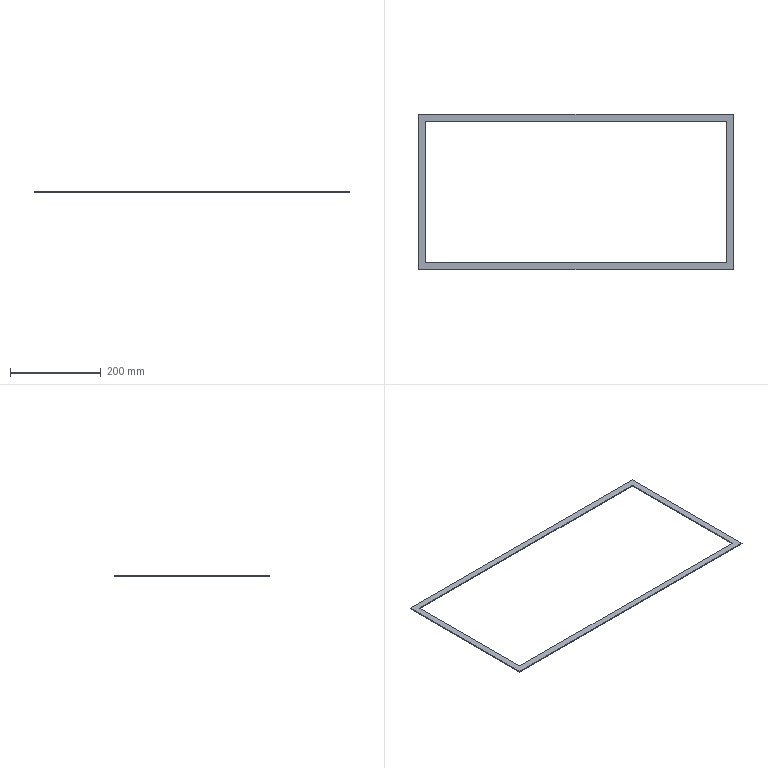Part | SolidWorks | features Extrusion 1 | 1 solid | 10 faces | box 692 x 342 x 2 mm | volume 60240 mm3 | plane 10
STEP:
#1=CARTESIAN_POINT('',(346.,-171.,1.));
#2=VERTEX_POINT('',#1);
#3=CARTESIAN_POINT('',(346.,171.,1.));
#4=VERTEX_POINT('',#3);
#5=CARTESIAN_POINT('',(346.,-171.,1.));
#6=DIRECTION('',(0.,1.,0.));
#7=VECTOR('',#6,1000.);
#8=LINE('',#5,#7);
#9=EDGE_CURVE('',#2,#4,#8,.T.);
#10=ORIENTED_EDGE('',*,*,#9,.T.);
#11=CARTESIAN_POINT('',(-346.,171.,1.));
#12=VERTEX_POINT('',#11);
#13=CARTESIAN_POINT('',(-346.,171.,1.));
#14=DIRECTION('',(-1.,0.,0.));
#15=VECTOR('',#14,1000.);
#16=LINE('',#13,#15);
#17=EDGE_CURVE('',#4,#12,#16,.T.);
#18=ORIENTED_EDGE('',*,*,#17,.T.);
#19=CARTESIAN_POINT('',(-346.,-171.,1.));
#20=VERTEX_POINT('',#19);
#21=CARTESIAN_POINT('',(-346.,-171.,1.));
#22=DIRECTION('',(0.,-1.,0.));
#23=VECTOR('',#22,1000.);
#24=LINE('',#21,#23);
#25=EDGE_CURVE('',#12,#20,#24,.T.);
#26=ORIENTED_EDGE('',*,*,#25,.T.);
#27=CARTESIAN_POINT('',(-346.,-171.,1.));
#28=DIRECTION('',(1.,0.,0.));
#29=VECTOR('',#28,1000.);
#30=LINE('',#27,#29);
#31=EDGE_CURVE('',#20,#2,#30,.T.);
#32=ORIENTED_EDGE('',*,*,#31,.T.);
#33=EDGE_LOOP('',(#10,#18,#26,#32));
#34=FACE_OUTER_BOUND('',#33,.T.);
#35=CARTESIAN_POINT('',(-331.,156.,1.));
#36=VERTEX_POINT('',#35);
#37=CARTESIAN_POINT('',(-331.,-156.,1.));
#38=VERTEX_POINT('',#37);
#39=CARTESIAN_POINT('',(-331.,-156.,1.));
#40=DIRECTION('',(0.,-1.,0.));
#41=VECTOR('',#40,1000.);
#42=LINE('',#39,#41);
#43=EDGE_CURVE('',#36,#38,#42,.T.);
#44=ORIENTED_EDGE('',*,*,#43,.F.);
#45=CARTESIAN_POINT('',(331.,156.,1.));
#46=VERTEX_POINT('',#45);
#47=CARTESIAN_POINT('',(-331.,156.,1.));
#48=DIRECTION('',(-1.,0.,0.));
#49=VECTOR('',#48,1000.);
#50=LINE('',#47,#49);
#51=EDGE_CURVE('',#46,#36,#50,.T.);
#52=ORIENTED_EDGE('',*,*,#51,.F.);
#53=CARTESIAN_POINT('',(331.,-156.,1.));
#54=VERTEX_POINT('',#53);
#55=CARTESIAN_POINT('',(331.,-156.,1.));
#56=DIRECTION('',(0.,1.,0.));
#57=VECTOR('',#56,1000.);
#58=LINE('',#55,#57);
#59=EDGE_CURVE('',#54,#46,#58,.T.);
#60=ORIENTED_EDGE('',*,*,#59,.F.);
#61=CARTESIAN_POINT('',(-331.,-156.,1.));
#62=DIRECTION('',(1.,0.,0.));
#63=VECTOR('',#62,1000.);
#64=LINE('',#61,#63);
#65=EDGE_CURVE('',#38,#54,#64,.T.);
#66=ORIENTED_EDGE('',*,*,#65,.F.);
#67=EDGE_LOOP('',(#44,#52,#60,#66));
#68=FACE_BOUND('',#67,.T.);
#69=CARTESIAN_POINT('',(0.,0.,1.));
#70=DIRECTION('',(0.,0.,-1.));
#71=DIRECTION('',(-1.,0.,0.));
#72=AXIS2_PLACEMENT_3D('',#69,#70,#71);
#73=PLANE('',#72);
#74=ADVANCED_FACE('',(#34,#68),#73,.F.);
#75=CARTESIAN_POINT('',(346.,-171.,-1.));
#76=VERTEX_POINT('',#75);
#77=CARTESIAN_POINT('',(346.,171.,-1.));
#78=VERTEX_POINT('',#77);
#79=CARTESIAN_POINT('',(346.,-171.,-1.));
#80=DIRECTION('',(0.,1.,0.));
#81=VECTOR('',#80,1000.);
#82=LINE('',#79,#81);
#83=EDGE_CURVE('',#76,#78,#82,.T.);
#84=ORIENTED_EDGE('',*,*,#83,.F.);
#85=CARTESIAN_POINT('',(-346.,-171.,-1.));
#86=VERTEX_POINT('',#85);
#87=CARTESIAN_POINT('',(-346.,-171.,-1.));
#88=DIRECTION('',(1.,0.,0.));
#89=VECTOR('',#88,1000.);
#90=LINE('',#87,#89);
#91=EDGE_CURVE('',#86,#76,#90,.T.);
#92=ORIENTED_EDGE('',*,*,#91,.F.);
#93=CARTESIAN_POINT('',(-346.,171.,-1.));
#94=VERTEX_POINT('',#93);
#95=CARTESIAN_POINT('',(-346.,-171.,-1.));
#96=DIRECTION('',(0.,-1.,0.));
#97=VECTOR('',#96,1000.);
#98=LINE('',#95,#97);
#99=EDGE_CURVE('',#94,#86,#98,.T.);
#100=ORIENTED_EDGE('',*,*,#99,.F.);
#101=CARTESIAN_POINT('',(-346.,171.,-1.));
#102=DIRECTION('',(-1.,0.,0.));
#103=VECTOR('',#102,1000.);
#104=LINE('',#101,#103);
#105=EDGE_CURVE('',#78,#94,#104,.T.);
#106=ORIENTED_EDGE('',*,*,#105,.F.);
#107=EDGE_LOOP('',(#84,#92,#100,#106));
#108=FACE_OUTER_BOUND('',#107,.T.);
#109=CARTESIAN_POINT('',(331.,156.,-1.));
#110=VERTEX_POINT('',#109);
#111=CARTESIAN_POINT('',(-331.,156.,-1.));
#112=VERTEX_POINT('',#111);
#113=CARTESIAN_POINT('',(-331.,156.,-1.));
#114=DIRECTION('',(-1.,0.,0.));
#115=VECTOR('',#114,1000.);
#116=LINE('',#113,#115);
#117=EDGE_CURVE('',#110,#112,#116,.T.);
#118=ORIENTED_EDGE('',*,*,#117,.T.);
#119=CARTESIAN_POINT('',(-331.,-156.,-1.));
#120=VERTEX_POINT('',#119);
#121=CARTESIAN_POINT('',(-331.,-156.,-1.));
#122=DIRECTION('',(0.,-1.,0.));
#123=VECTOR('',#122,1000.);
#124=LINE('',#121,#123);
#125=EDGE_CURVE('',#112,#120,#124,.T.);
#126=ORIENTED_EDGE('',*,*,#125,.T.);
#127=CARTESIAN_POINT('',(331.,-156.,-1.));
#128=VERTEX_POINT('',#127);
#129=CARTESIAN_POINT('',(-331.,-156.,-1.));
#130=DIRECTION('',(1.,0.,0.));
#131=VECTOR('',#130,1000.);
#132=LINE('',#129,#131);
#133=EDGE_CURVE('',#120,#128,#132,.T.);
#134=ORIENTED_EDGE('',*,*,#133,.T.);
#135=CARTESIAN_POINT('',(331.,-156.,-1.));
#136=DIRECTION('',(0.,1.,0.));
#137=VECTOR('',#136,1000.);
#138=LINE('',#135,#137);
#139=EDGE_CURVE('',#128,#110,#138,.T.);
#140=ORIENTED_EDGE('',*,*,#139,.T.);
#141=EDGE_LOOP('',(#118,#126,#134,#140));
#142=FACE_BOUND('',#141,.T.);
#143=CARTESIAN_POINT('',(0.,0.,-1.));
#144=DIRECTION('',(0.,0.,-1.));
#145=DIRECTION('',(-1.,0.,0.));
#146=AXIS2_PLACEMENT_3D('',#143,#144,#145);
#147=PLANE('',#146);
#148=ADVANCED_FACE('',(#108,#142),#147,.T.);
#149=ORIENTED_EDGE('',*,*,#83,.T.);
#150=CARTESIAN_POINT('',(346.,171.,1.));
#151=DIRECTION('',(0.,0.,-1.));
#152=VECTOR('',#151,1000.);
#153=LINE('',#150,#152);
#154=EDGE_CURVE('',#4,#78,#153,.T.);
#155=ORIENTED_EDGE('',*,*,#154,.F.);
#156=ORIENTED_EDGE('',*,*,#9,.F.);
#157=CARTESIAN_POINT('',(346.,-171.,1.));
#158=DIRECTION('',(0.,0.,-1.));
#159=VECTOR('',#158,1000.);
#160=LINE('',#157,#159);
#161=EDGE_CURVE('',#2,#76,#160,.T.);
#162=ORIENTED_EDGE('',*,*,#161,.T.);
#163=EDGE_LOOP('',(#149,#155,#156,#162));
#164=FACE_OUTER_BOUND('',#163,.T.);
#165=CARTESIAN_POINT('',(346.,-171.,1.));
#166=DIRECTION('',(-1.,0.,0.));
#167=DIRECTION('',(0.,0.,1.));
#168=AXIS2_PLACEMENT_3D('',#165,#166,#167);
#169=PLANE('',#168);
#170=ADVANCED_FACE('',(#164),#169,.F.);
#171=ORIENTED_EDGE('',*,*,#105,.T.);
#172=CARTESIAN_POINT('',(-346.,171.,1.));
#173=DIRECTION('',(0.,0.,-1.));
#174=VECTOR('',#173,1000.);
#175=LINE('',#172,#174);
#176=EDGE_CURVE('',#12,#94,#175,.T.);
#177=ORIENTED_EDGE('',*,*,#176,.F.);
#178=ORIENTED_EDGE('',*,*,#17,.F.);
#179=ORIENTED_EDGE('',*,*,#154,.T.);
#180=EDGE_LOOP('',(#171,#177,#178,#179));
#181=FACE_OUTER_BOUND('',#180,.T.);
#182=CARTESIAN_POINT('',(-346.,171.,1.));
#183=DIRECTION('',(0.,-1.,0.));
#184=DIRECTION('',(0.,0.,-1.));
#185=AXIS2_PLACEMENT_3D('',#182,#183,#184);
#186=PLANE('',#185);
#187=ADVANCED_FACE('',(#181),#186,.F.);
#188=ORIENTED_EDGE('',*,*,#99,.T.);
#189=CARTESIAN_POINT('',(-346.,-171.,1.));
#190=DIRECTION('',(0.,0.,-1.));
#191=VECTOR('',#190,1000.);
#192=LINE('',#189,#191);
#193=EDGE_CURVE('',#20,#86,#192,.T.);
#194=ORIENTED_EDGE('',*,*,#193,.F.);
#195=ORIENTED_EDGE('',*,*,#25,.F.);
#196=ORIENTED_EDGE('',*,*,#176,.T.);
#197=EDGE_LOOP('',(#188,#194,#195,#196));
#198=FACE_OUTER_BOUND('',#197,.T.);
#199=CARTESIAN_POINT('',(-346.,-171.,1.));
#200=DIRECTION('',(1.,0.,0.));
#201=DIRECTION('',(0.,0.,-1.));
#202=AXIS2_PLACEMENT_3D('',#199,#200,#201);
#203=PLANE('',#202);
#204=ADVANCED_FACE('',(#198),#203,.F.);
#205=ORIENTED_EDGE('',*,*,#91,.T.);
#206=ORIENTED_EDGE('',*,*,#161,.F.);
#207=ORIENTED_EDGE('',*,*,#31,.F.);
#208=ORIENTED_EDGE('',*,*,#193,.T.);
#209=EDGE_LOOP('',(#205,#206,#207,#208));
#210=FACE_OUTER_BOUND('',#209,.T.);
#211=CARTESIAN_POINT('',(-346.,-171.,1.));
#212=DIRECTION('',(0.,1.,0.));
#213=DIRECTION('',(0.,0.,1.));
#214=AXIS2_PLACEMENT_3D('',#211,#212,#213);
#215=PLANE('',#214);
#216=ADVANCED_FACE('',(#210),#215,.F.);
#217=ORIENTED_EDGE('',*,*,#125,.F.);
#218=CARTESIAN_POINT('',(-331.,156.,1.));
#219=DIRECTION('',(0.,0.,-1.));
#220=VECTOR('',#219,1000.);
#221=LINE('',#218,#220);
#222=EDGE_CURVE('',#36,#112,#221,.T.);
#223=ORIENTED_EDGE('',*,*,#222,.F.);
#224=ORIENTED_EDGE('',*,*,#43,.T.);
#225=CARTESIAN_POINT('',(-331.,-156.,1.));
#226=DIRECTION('',(0.,0.,-1.));
#227=VECTOR('',#226,1000.);
#228=LINE('',#225,#227);
#229=EDGE_CURVE('',#38,#120,#228,.T.);
#230=ORIENTED_EDGE('',*,*,#229,.T.);
#231=EDGE_LOOP('',(#217,#223,#224,#230));
#232=FACE_OUTER_BOUND('',#231,.T.);
#233=CARTESIAN_POINT('',(-331.,-156.,1.));
#234=DIRECTION('',(1.,0.,0.));
#235=DIRECTION('',(0.,0.,-1.));
#236=AXIS2_PLACEMENT_3D('',#233,#234,#235);
#237=PLANE('',#236);
#238=ADVANCED_FACE('',(#232),#237,.T.);
#239=ORIENTED_EDGE('',*,*,#133,.F.);
#240=ORIENTED_EDGE('',*,*,#229,.F.);
#241=ORIENTED_EDGE('',*,*,#65,.T.);
#242=CARTESIAN_POINT('',(331.,-156.,1.));
#243=DIRECTION('',(0.,0.,-1.));
#244=VECTOR('',#243,1000.);
#245=LINE('',#242,#244);
#246=EDGE_CURVE('',#54,#128,#245,.T.);
#247=ORIENTED_EDGE('',*,*,#246,.T.);
#248=EDGE_LOOP('',(#239,#240,#241,#247));
#249=FACE_OUTER_BOUND('',#248,.T.);
#250=CARTESIAN_POINT('',(-331.,-156.,1.));
#251=DIRECTION('',(0.,1.,0.));
#252=DIRECTION('',(0.,0.,1.));
#253=AXIS2_PLACEMENT_3D('',#250,#251,#252);
#254=PLANE('',#253);
#255=ADVANCED_FACE('',(#249),#254,.T.);
#256=ORIENTED_EDGE('',*,*,#139,.F.);
#257=ORIENTED_EDGE('',*,*,#246,.F.);
#258=ORIENTED_EDGE('',*,*,#59,.T.);
#259=CARTESIAN_POINT('',(331.,156.,1.));
#260=DIRECTION('',(0.,0.,-1.));
#261=VECTOR('',#260,1000.);
#262=LINE('',#259,#261);
#263=EDGE_CURVE('',#46,#110,#262,.T.);
#264=ORIENTED_EDGE('',*,*,#263,.T.);
#265=EDGE_LOOP('',(#256,#257,#258,#264));
#266=FACE_OUTER_BOUND('',#265,.T.);
#267=CARTESIAN_POINT('',(331.,-156.,1.));
#268=DIRECTION('',(-1.,0.,0.));
#269=DIRECTION('',(0.,0.,1.));
#270=AXIS2_PLACEMENT_3D('',#267,#268,#269);
#271=PLANE('',#270);
#272=ADVANCED_FACE('',(#266),#271,.T.);
#273=ORIENTED_EDGE('',*,*,#117,.F.);
#274=ORIENTED_EDGE('',*,*,#263,.F.);
#275=ORIENTED_EDGE('',*,*,#51,.T.);
#276=ORIENTED_EDGE('',*,*,#222,.T.);
#277=EDGE_LOOP('',(#273,#274,#275,#276));
#278=FACE_OUTER_BOUND('',#277,.T.);
#279=CARTESIAN_POINT('',(-331.,156.,1.));
#280=DIRECTION('',(0.,-1.,0.));
#281=DIRECTION('',(1.,0.,0.));
#282=AXIS2_PLACEMENT_3D('',#279,#280,#281);
#283=PLANE('',#282);
#284=ADVANCED_FACE('',(#278),#283,.T.);
#285=CLOSED_SHELL('',(#74,#148,#170,#187,#204,#216,#238,#255,#272,#284));
#286=MANIFOLD_SOLID_BREP('',#285);
#287=CARTESIAN_POINT('',(0.,0.,0.));
#288=DIRECTION('',(0.,0.,1.));
#289=DIRECTION('',(1.,0.,0.));
#290=AXIS2_PLACEMENT_3D('',#287,#288,#289);
#291=(LENGTH_UNIT()NAMED_UNIT(*)SI_UNIT(.MILLI.,.METRE.));
#292=UNCERTAINTY_MEASURE_WITH_UNIT(LENGTH_MEASURE(0.00001),#291,'','');
#293=(NAMED_UNIT(*)PLANE_ANGLE_UNIT()SI_UNIT($,.RADIAN.));
#294=(NAMED_UNIT(*)SI_UNIT($,.STERADIAN.)SOLID_ANGLE_UNIT());
#295=(GEOMETRIC_REPRESENTATION_CONTEXT(3)GLOBAL_UNCERTAINTY_ASSIGNED_CONTEXT((#292))GLOBAL_UNIT_ASSIGNED_CONTEXT((#291,#293,#294))REPRESENTATION_CONTEXT('',''));
#296=ADVANCED_BREP_SHAPE_REPRESENTATION('',(#286,#290),#295);